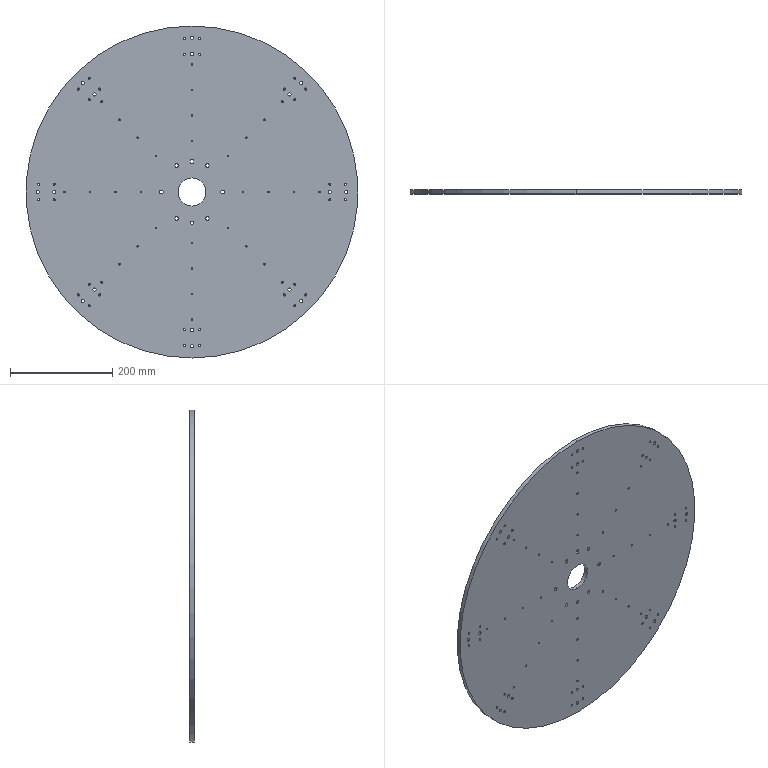Part | STEP file | 10-01 turntable | 1 solid | 185 faces | box 650 x 8 x 650 mm | volume 2623771 mm3 | cylinder 181 | plane 4 | commonest cylinder face diameters 3.3 x64 4.2 x64 6 x37 7 x12 55.1 x2 650 x2